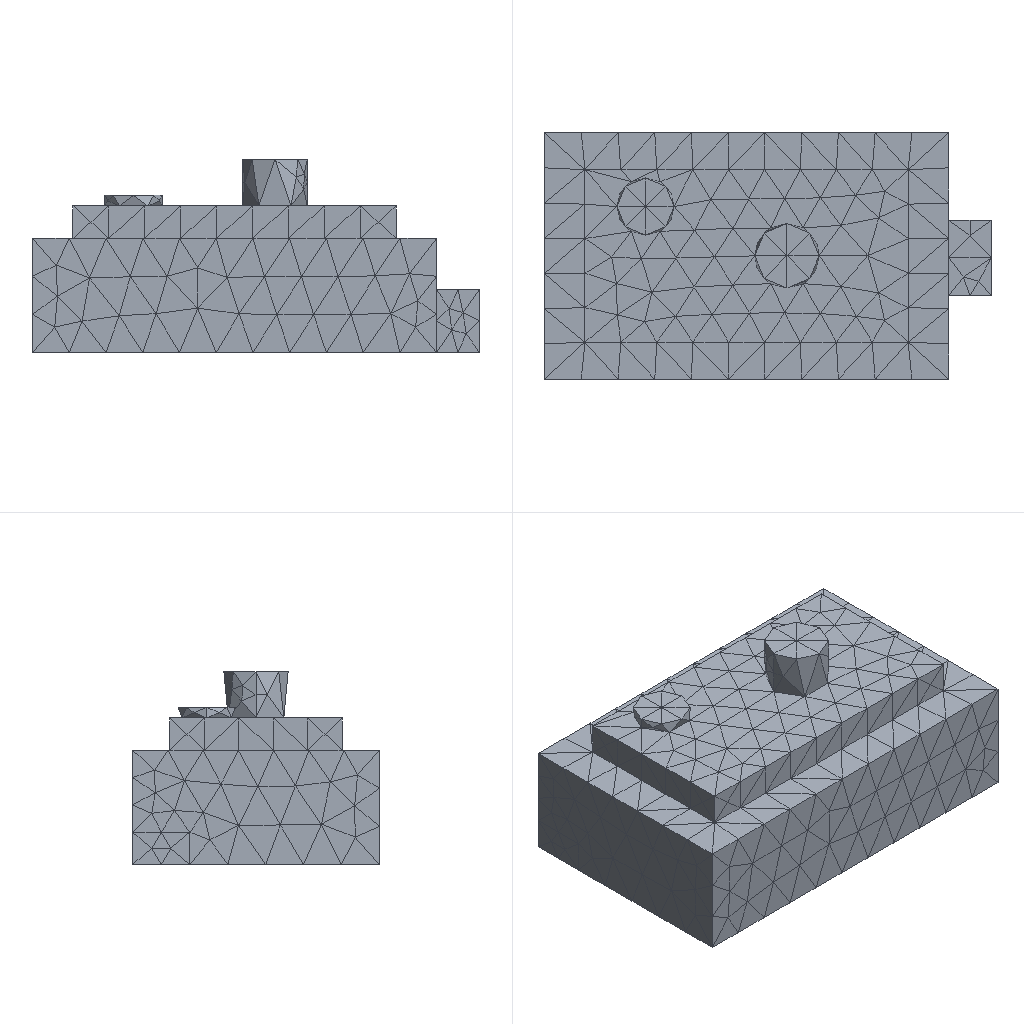Simulation study | ansys mapdl
Set-up summary:
category,name,step,type,value,unit,region
solver,ansys_mapdl
units,mm-N-s-tonne (MPa),,inferred,E=210000 density=
analysis,model,,static
mesh,nodes,,,4090
mesh,elements,,,2404
element_type,SOLID187,,,2404
material,mat 1,,E,210000
material,mat 1,,nu,0.3
load,,model,body load temp,,,all
load,,model,force,"1000 [dir=(0, 0, -1) n=146]",,node list
bc,,model,fixed,"[dofs=UX,UY,UZ n=4439]",,node list
Ansys APDL input file, long lists of numbers shortened:
/COM,ANSYS RELEASE 2026 R1           BUILD 26.1      UP20260202       09:09:22
/PREP7
/NOPR
/TITLE,2
ANTYPE, 0
*IF,_CDRDOFF,EQ,1,THEN     !if solid model was read in
_CDRDOFF=             !reset flag, numoffs already performed
*ELSE              !offset database for the following FE model
NUMOFF,NODE,     4090
NUMOFF,ELEM,     2404
NUMOFF,MAT ,        1
NUMOFF,TYPE,        1
*ENDIF
*SET,_RETURN ,  0.
*SET,_STATUS ,  0.
*SET,_UIQR   ,  146.
*SET,__FLOATPARAMETER__,  4090.
DOF,DELETE
ETBLOCK,        1,        1
(2i9,19a9)
        1      187        0        0        0        0        0        0        0        0        0        0        0        0        0        0        0        0        0        0        0
       -1
NBLOCK,6,SOLID,      4090,      4090
(3i9,6e21.13e3)
        1        0        0-4.0550000000000E+001 3.4500000000000E+001 9.0000000000000E+000
! (4089 more lines like these left out)
N,UNBL,LOC,       -1,
EBLOCK,19,SOLID,      2404,      2404
(19i10)
         1         1         1         1         0         0         0         0        10         0         1      1671      1672      1673      1674      1887      1888      1889      1890
! (4807 more lines like these left out)
        -1
MPTEMP,UNBL, 1, 1,  0.    ,
MPDATA,UNBL, 1,EX  ,       1, 1,  210000.000    ,
MPTEMP,UNBL, 1, 1,  0.    ,
MPDATA,UNBL, 1,NUXY,       1, 1, 0.3    ,
MPTEMP,UNBL, 1, 1,  0.    ,
MPDATA,UNBL, 1,PRXY,       1, 1, 0.3    ,
EXTOPT,ATTR,      0,      0,      0
EXTOPT,ESIZE,  0,  0.
EXTOPT,ACLEAR,      0
TREF,  0.
IRLF,  0
BFUNIF,TEMP,_TINY
ACEL,  0.    ,  0.    ,  0.
OMEGA,  0.    ,  0.    ,  0.
DOMEGA,  0.    ,  0.    ,  0.
CGLOC,  0.    ,  0.    ,  0.
CGOMEGA,  0.    ,  0.    ,  0.
DCGOMG,  0.    ,  0.    ,  0.
KUSE,     0
TIME,  0.
ALPHAD,  0.
BETAD,  0.
DMPRAT,  0.
DMPSTR,  0.
CRPLIM, 0.1    ,   0
CRPLIM,  0.    ,   1
NCNV,     0, 1.000000000E+12,     0,  0.    ,  0.
NEQIT,     0
ERESX,DEFA
DBLOCK,      4439
(i9,a6,2(pg16.9))
        1  UX    0.00000000      0.00000000
! (4438 more lines like these left out)
       -1
FBLOCK,       146
(i9,a6,2(pg16.9))
      865  FZ   -6.84931507      0.00000000
! (145 more lines like these left out)
       -1
/GO
FINISH
Results summary:
result,analysis_type_db,,,static,unstated
result,n_sets,,,1,unstated
result,load_steps[0].set,load_step=1,,1,unstated
result,load_steps[0].substep,load_step=1,,1,unstated
result,load_steps[0].time,load_step=1,,1,unstated
result,load_steps[0].freq,load_step=1,,1,unstated
result,load_steps[0].max_usum,load_step=1,,0.0004089,unstated
result,load_steps[0].max_seqv,load_step=1,,5.483,unstated
result,load_steps[0].reaction_sum.FX,load_step=1,,7.56788e-12,unstated
result,load_steps[0].reaction_sum.FY,load_step=1,,-5.29169e-12,unstated
result,load_steps[0].reaction_sum.FZ,load_step=1,,1000,unstated
result,load_steps[0].reaction_sum.MX,load_step=1,,0,unstated
result,load_steps[0].reaction_sum.MY,load_step=1,,0,unstated
result,load_steps[0].reaction_sum.MZ,load_step=1,,0,unstated
result,convergence,,,results present for all listed sets,unstated